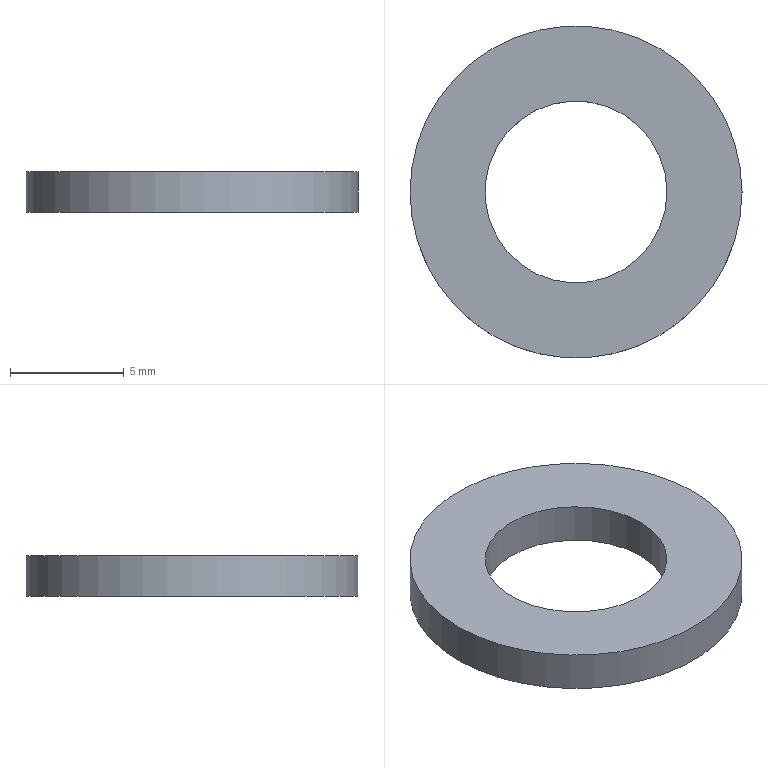Part | NX | features solid 2 | 1 solid | 4 faces | box 14.6 x 14.6 x 1.8 mm | volume 210.87 mm3 | plane 2 | cylinder 2 | commonest cylinder face diameters 8 x1 14.6 x1
STEP:
#1=CARTESIAN_POINT('',(-81.,30.,80.));
#2=VERTEX_POINT('',#1);
#3=CARTESIAN_POINT('',(-85.,30.,80.));
#4=DIRECTION('',(0.,0.,1.));
#5=DIRECTION('',(1.,0.,0.));
#6=AXIS2_PLACEMENT_3D('',#3,#4,#5);
#7=CIRCLE('',#6,4.);
#8=EDGE_CURVE('',#2,#2,#7,.T.);
#9=ORIENTED_EDGE('',*,*,#8,.T.);
#10=EDGE_LOOP('',(#9));
#11=FACE_BOUND('',#10,.T.);
#12=CARTESIAN_POINT('',(-77.7,30.,80.));
#13=VERTEX_POINT('',#12);
#14=CARTESIAN_POINT('',(-85.,30.,80.));
#15=DIRECTION('',(0.,0.,1.));
#16=DIRECTION('',(1.,0.,0.));
#17=AXIS2_PLACEMENT_3D('',#14,#15,#16);
#18=CIRCLE('',#17,7.3);
#19=EDGE_CURVE('',#13,#13,#18,.T.);
#20=ORIENTED_EDGE('',*,*,#19,.F.);
#21=EDGE_LOOP('',(#20));
#22=FACE_BOUND('',#21,.T.);
#23=CARTESIAN_POINT('',(-92.3,30.,80.));
#24=DIRECTION('',(0.,0.,-1.));
#25=DIRECTION('',(-1.,0.,0.));
#26=AXIS2_PLACEMENT_3D('',#23,#24,#25);
#27=PLANE('',#26);
#28=ADVANCED_FACE('',(#11,#22),#27,.T.);
#29=CARTESIAN_POINT('',(-81.,30.,81.8));
#30=VERTEX_POINT('',#29);
#31=CARTESIAN_POINT('',(-85.,30.,81.8));
#32=DIRECTION('',(0.,0.,1.));
#33=DIRECTION('',(1.,0.,0.));
#34=AXIS2_PLACEMENT_3D('',#31,#32,#33);
#35=CIRCLE('',#34,4.);
#36=EDGE_CURVE('',#30,#30,#35,.T.);
#37=ORIENTED_EDGE('',*,*,#36,.T.);
#38=EDGE_LOOP('',(#37));
#39=FACE_BOUND('',#38,.T.);
#40=ORIENTED_EDGE('',*,*,#8,.F.);
#41=EDGE_LOOP('',(#40));
#42=FACE_BOUND('',#41,.T.);
#43=CARTESIAN_POINT('',(-85.,30.,80.));
#44=DIRECTION('',(0.,0.,1.));
#45=DIRECTION('',(1.,0.,0.));
#46=AXIS2_PLACEMENT_3D('',#43,#44,#45);
#47=CYLINDRICAL_SURFACE('',#46,4.);
#48=ADVANCED_FACE('',(#39,#42),#47,.F.);
#49=CARTESIAN_POINT('',(-77.7,30.,81.8));
#50=VERTEX_POINT('',#49);
#51=CARTESIAN_POINT('',(-85.,30.,81.8));
#52=DIRECTION('',(0.,0.,1.));
#53=DIRECTION('',(1.,0.,0.));
#54=AXIS2_PLACEMENT_3D('',#51,#52,#53);
#55=CIRCLE('',#54,7.3);
#56=EDGE_CURVE('',#50,#50,#55,.T.);
#57=ORIENTED_EDGE('',*,*,#56,.T.);
#58=EDGE_LOOP('',(#57));
#59=FACE_BOUND('',#58,.T.);
#60=ORIENTED_EDGE('',*,*,#36,.F.);
#61=EDGE_LOOP('',(#60));
#62=FACE_BOUND('',#61,.T.);
#63=CARTESIAN_POINT('',(-89.,30.,81.8));
#64=DIRECTION('',(0.,0.,1.));
#65=DIRECTION('',(1.,0.,0.));
#66=AXIS2_PLACEMENT_3D('',#63,#64,#65);
#67=PLANE('',#66);
#68=ADVANCED_FACE('',(#59,#62),#67,.T.);
#69=ORIENTED_EDGE('',*,*,#19,.T.);
#70=EDGE_LOOP('',(#69));
#71=FACE_BOUND('',#70,.T.);
#72=ORIENTED_EDGE('',*,*,#56,.F.);
#73=EDGE_LOOP('',(#72));
#74=FACE_BOUND('',#73,.T.);
#75=CARTESIAN_POINT('',(-85.,30.,80.));
#76=DIRECTION('',(0.,0.,1.));
#77=DIRECTION('',(1.,0.,0.));
#78=AXIS2_PLACEMENT_3D('',#75,#76,#77);
#79=CYLINDRICAL_SURFACE('',#78,7.3);
#80=ADVANCED_FACE('',(#71,#74),#79,.T.);
#81=CLOSED_SHELL('',(#28,#48,#68,#80));
#82=MANIFOLD_SOLID_BREP('',#81);
#83=(LENGTH_UNIT()NAMED_UNIT(*)SI_UNIT(.MILLI.,.METRE.));
#84=UNCERTAINTY_MEASURE_WITH_UNIT(LENGTH_MEASURE(0.00001),#83,'','');
#85=(NAMED_UNIT(*)PLANE_ANGLE_UNIT()SI_UNIT($,.RADIAN.));
#86=(NAMED_UNIT(*)SI_UNIT($,.STERADIAN.)SOLID_ANGLE_UNIT());
#87=(GEOMETRIC_REPRESENTATION_CONTEXT(3)GLOBAL_UNCERTAINTY_ASSIGNED_CONTEXT((#84))GLOBAL_UNIT_ASSIGNED_CONTEXT((#83,#85,#86))REPRESENTATION_CONTEXT('',''));
#88=ADVANCED_BREP_SHAPE_REPRESENTATION('',(#82),#87);